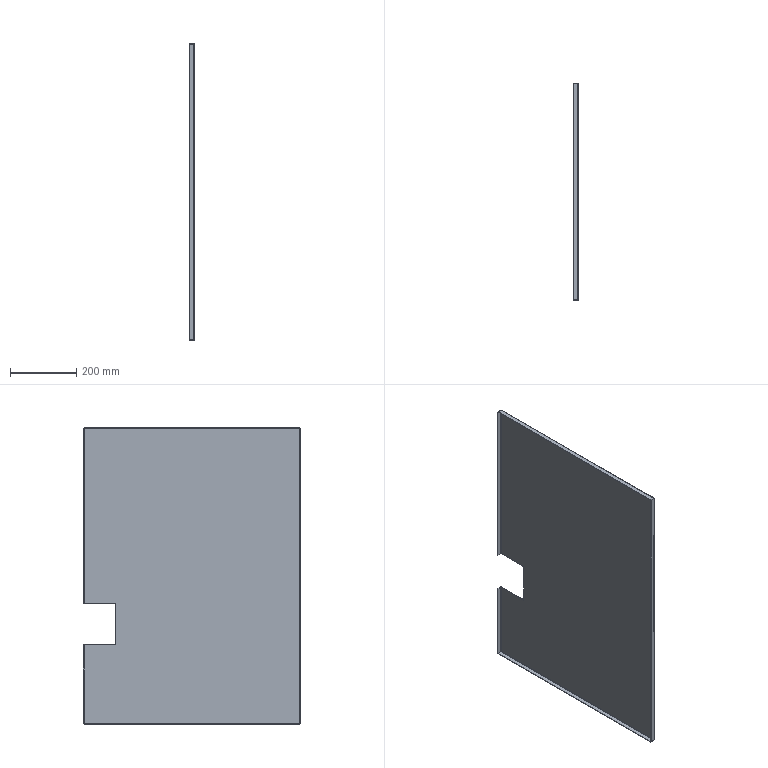Part | SolidWorks | features BaseBody 1 | 1 solid | 46 faces | box 15 x 658 x 898 mm | volume 925138 mm3 | plane 28 | cylinder 10 | spline 8 | commonest cylinder face diameters 1.473 x5 4.473 x5